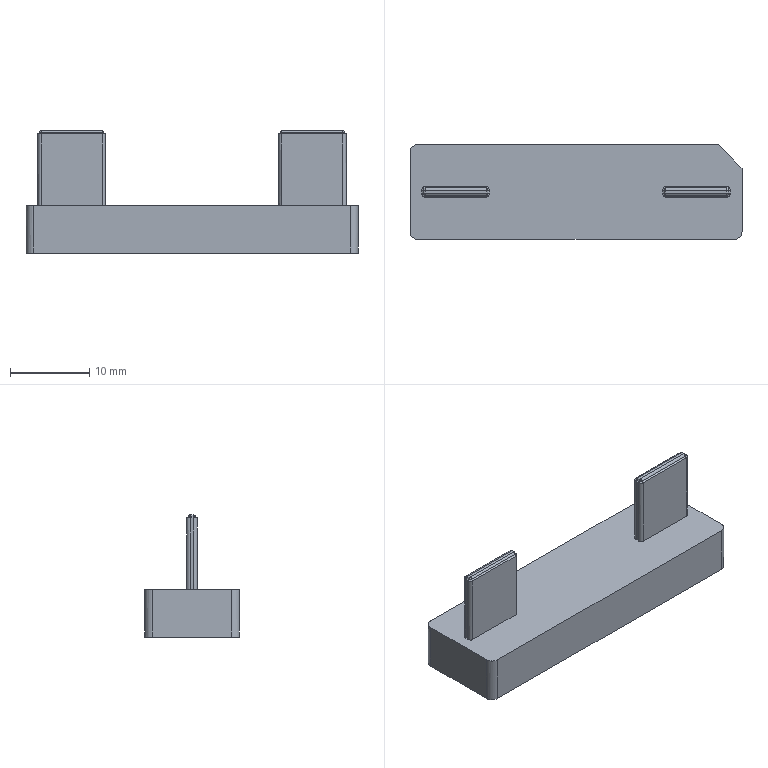CAM job | PowerMill | 3-axis milling, other | part box 42 x 12 x 15.447 mm
Tools:
number,name,type,diameter,tip_radius,length,cutting_length,overhang,flutes,holder,toolpaths_using
1,D10C,end_mill,10.0,0.0,60.0,,30.0,1,D42L35,1
1,D10C_1_1,end_mill,10.0,0.0,60.0,,15.88,1,D42L35,3
2,D4C_1_1,end_mill,4.0,0.0,30.0,,9.64,1,D42L35,1
3,D10_1_1,end_mill,10.0,0.0,60.0,,15.6,1,D42L35,3
14,D4_1_1,end_mill,4.0,0.0,30.0,,9.6,1,D42L35,2
13,Text_D4_1_1,taper_spherical,4.0,0.3,60.0,,9.72,1,D42L35,1
Operations:
program,toolpath,strategy,tool,tool_number,tool_diameter,tip_radius,flutes,spindle_rpm,feed_cut,surface_speed_m_min_computed,feed_per_tooth_computed,tolerance,thickness,stepover,stepdown,cut_length,cut_time_min,total_time_min,workplane
16-0919-1-F,精公开粗01-扫面平行-D10C,raster_area_clear,D10C_1_1,1,10.0,0.0,1.0,8000.0,10000.0,251.33,1.25,0.03,0.28,6.0,1.0,207.8,0.021,0.0269,
16-0919-1-F,精公开粗01-外形偏置-D10C,offset_area_clear,D10C_1_1,1,10.0,0.0,1.0,8000.0,10000.0,251.33,1.25,0.03,0.28,6.0,1.0,6943.195,0.694,0.7564,
16-0919-1-F,精公开粗01-基准台等高-D10C,constantz,D10C_1_1,1,10.0,0.0,1.0,8000.0,10000.0,251.33,1.25,0.03,0.07,5.0,0.4,2325.127,0.233,0.2419,
16-0919-1-F,精公再粗02-外形偏置-D4C,offset_area_clear,D4C_1_1,2,4.0,0.0,1.0,18000.0,6000.0,226.19,0.3333,0.03,0.0,2.0,1.0,3350.072,0.558,0.6079,
16-0919-1-F,精公基准台01-平坦面平行-D10,raster_area_clear,D10_1_1,3,10.0,0.0,1.0,8500.0,600.0,267.04,0.0706,0.005,0.38,5.0,1.0,80.663,0.134,0.1657,
16-0919-1-F,精公基准台01-基准面偏置-D10,offset_area_clear,D10_1_1,3,10.0,0.0,1.0,8500.0,600.0,267.04,0.0706,0.005,0.38,5.0,1.0,157.289,0.262,0.3015,
16-0919-1-F,精公基准台01-基准台侧光-D10,profile_area_clear,D10_1_1,3,10.0,0.0,1.0,8500.0,600.0,267.04,0.0706,0.005,0.0,0.08,1.0,273.234,0.455,0.5191,
16-0919-1-F,精公精光01-等高-D4,constantz,D4_1_1,14,4.0,0.0,1.0,18000.0,2000.0,226.19,0.1111,0.005,-0.075,5.0,0.01,16383.208,8.192,8.208,
16-0919-1-F,精公精光01-平坦面平行-D4,raster_area_clear,D4_1_1,14,4.0,0.0,1.0,18000.0,600.0,226.19,0.0333,0.005,0.375,2.0,1.0,53.929,0.09,0.1106,
16-0919-1-F,精公刻字01-刻字-Text_D4,pattern,Text_D4_1_1,13,4.0,0.3,1.0,15000.0,1000.0,188.5,0.0667,0.005,0.0,5.0,1.0,63.388,0.063,0.0839,
,精公开粗01-外形偏置-D10C-02_Reference,offset_area_clear,D10C,1,10.0,0.0,1.0,8000.0,10000.0,251.33,1.25,0.03,0.28,6.0,1.0,13604.506,1.36,1.478,